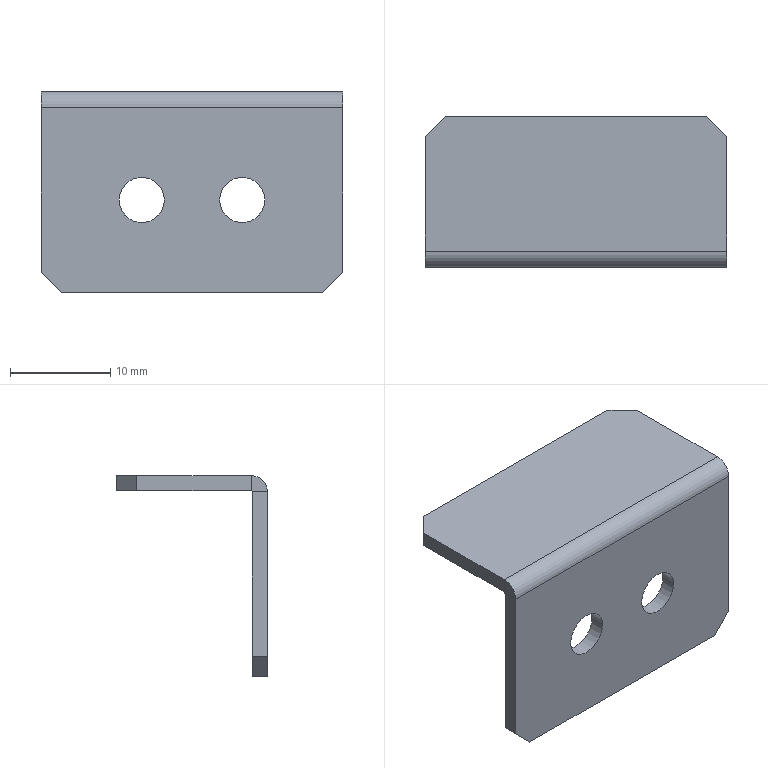Part | SolidWorks | features Chamfer 1, ICE 1, SplitBody 1 | 1 solid | 22 faces | box 30 x 15 x 20 mm | volume 1431 mm3 | plane 16 | cylinder 6 | commonest cylinder face diameters 4.5 x4 0.2 x1 3.2 x1
STEP:
#1=CARTESIAN_POINT('',(23.95,17.2,288.));
#2=VERTEX_POINT('',#1);
#3=CARTESIAN_POINT('',(19.45,17.2,288.));
#4=VERTEX_POINT('',#3);
#5=CARTESIAN_POINT('',(21.7,17.2,288.));
#6=DIRECTION('',(0.,1.,0.));
#7=DIRECTION('',(-1.,0.,0.));
#8=AXIS2_PLACEMENT_3D('',#5,#6,#7);
#9=CIRCLE('',#8,2.25);
#10=EDGE_CURVE('',#2,#4,#9,.T.);
#11=ORIENTED_EDGE('',*,*,#10,.F.);
#12=CARTESIAN_POINT('',(23.95,18.7,288.));
#13=VERTEX_POINT('',#12);
#14=CARTESIAN_POINT('',(23.95,8.7,288.));
#15=DIRECTION('',(0.,1.,0.));
#16=VECTOR('',#15,1000.);
#17=LINE('',#14,#16);
#18=EDGE_CURVE('',#2,#13,#17,.T.);
#19=ORIENTED_EDGE('',*,*,#18,.T.);
#20=CARTESIAN_POINT('',(19.45,18.7,288.));
#21=VERTEX_POINT('',#20);
#22=CARTESIAN_POINT('',(21.7,18.7,288.));
#23=DIRECTION('',(0.,1.,0.));
#24=DIRECTION('',(-1.,0.,0.));
#25=AXIS2_PLACEMENT_3D('',#22,#23,#24);
#26=CIRCLE('',#25,2.25);
#27=EDGE_CURVE('',#13,#21,#26,.T.);
#28=ORIENTED_EDGE('',*,*,#27,.T.);
#29=CARTESIAN_POINT('',(19.45,8.7,288.));
#30=DIRECTION('',(0.,1.,0.));
#31=VECTOR('',#30,1000.);
#32=LINE('',#29,#31);
#33=EDGE_CURVE('',#4,#21,#32,.T.);
#34=ORIENTED_EDGE('',*,*,#33,.F.);
#35=EDGE_LOOP('',(#11,#19,#28,#34));
#36=FACE_OUTER_BOUND('',#35,.T.);
#37=CARTESIAN_POINT('',(21.7,8.7,288.));
#38=DIRECTION('',(0.,1.,0.));
#39=DIRECTION('',(-1.,0.,0.));
#40=AXIS2_PLACEMENT_3D('',#37,#38,#39);
#41=CYLINDRICAL_SURFACE('',#40,2.25);
#42=ADVANCED_FACE('',(#36),#41,.F.);
#43=CARTESIAN_POINT('',(13.95,18.7,288.));
#44=VERTEX_POINT('',#43);
#45=CARTESIAN_POINT('',(9.45,18.7,288.));
#46=VERTEX_POINT('',#45);
#47=CARTESIAN_POINT('',(11.7,18.7,288.));
#48=DIRECTION('',(0.,-1.,0.));
#49=DIRECTION('',(1.,0.,0.));
#50=AXIS2_PLACEMENT_3D('',#47,#48,#49);
#51=CIRCLE('',#50,2.25);
#52=EDGE_CURVE('',#44,#46,#51,.T.);
#53=ORIENTED_EDGE('',*,*,#52,.F.);
#54=CARTESIAN_POINT('',(13.95,17.2,288.));
#55=VERTEX_POINT('',#54);
#56=CARTESIAN_POINT('',(13.95,22.2,288.));
#57=DIRECTION('',(0.,-1.,0.));
#58=VECTOR('',#57,1000.);
#59=LINE('',#56,#58);
#60=EDGE_CURVE('',#44,#55,#59,.T.);
#61=ORIENTED_EDGE('',*,*,#60,.T.);
#62=CARTESIAN_POINT('',(9.45,17.2,288.));
#63=VERTEX_POINT('',#62);
#64=CARTESIAN_POINT('',(11.7,17.2,288.));
#65=DIRECTION('',(0.,1.,0.));
#66=DIRECTION('',(-1.,0.,0.));
#67=AXIS2_PLACEMENT_3D('',#64,#65,#66);
#68=CIRCLE('',#67,2.25);
#69=EDGE_CURVE('',#63,#55,#68,.T.);
#70=ORIENTED_EDGE('',*,*,#69,.F.);
#71=CARTESIAN_POINT('',(9.45,22.2,288.));
#72=DIRECTION('',(0.,-1.,0.));
#73=VECTOR('',#72,1000.);
#74=LINE('',#71,#73);
#75=EDGE_CURVE('',#46,#63,#74,.T.);
#76=ORIENTED_EDGE('',*,*,#75,.F.);
#77=EDGE_LOOP('',(#53,#61,#70,#76));
#78=FACE_OUTER_BOUND('',#77,.T.);
#79=CARTESIAN_POINT('',(11.7,22.2,288.));
#80=DIRECTION('',(0.,-1.,0.));
#81=DIRECTION('',(-1.,0.,0.));
#82=AXIS2_PLACEMENT_3D('',#79,#80,#81);
#83=CYLINDRICAL_SURFACE('',#82,2.25);
#84=ADVANCED_FACE('',(#78),#83,.F.);
#85=CARTESIAN_POINT('',(31.7,17.2,297.2));
#86=VERTEX_POINT('',#85);
#87=CARTESIAN_POINT('',(31.7,18.7,297.2));
#88=VERTEX_POINT('',#87);
#89=CARTESIAN_POINT('',(31.7,17.2,297.2));
#90=DIRECTION('',(0.,1.,0.));
#91=VECTOR('',#90,1000.);
#92=LINE('',#89,#91);
#93=EDGE_CURVE('',#86,#88,#92,.T.);
#94=ORIENTED_EDGE('',*,*,#93,.T.);
#95=CARTESIAN_POINT('',(31.7,18.8,297.3));
#96=VERTEX_POINT('',#95);
#97=CARTESIAN_POINT('',(31.7,18.8,297.2));
#98=DIRECTION('',(-1.,0.,0.));
#99=DIRECTION('',(0.,0.,-1.));
#100=AXIS2_PLACEMENT_3D('',#97,#98,#99);
#101=CIRCLE('',#100,0.1);
#102=EDGE_CURVE('',#88,#96,#101,.T.);
#103=ORIENTED_EDGE('',*,*,#102,.T.);
#104=CARTESIAN_POINT('',(31.7,18.8,298.8));
#105=VERTEX_POINT('',#104);
#106=CARTESIAN_POINT('',(31.7,18.8,297.3));
#107=DIRECTION('',(0.,0.,1.));
#108=VECTOR('',#107,1000.);
#109=LINE('',#106,#108);
#110=EDGE_CURVE('',#96,#105,#109,.T.);
#111=ORIENTED_EDGE('',*,*,#110,.T.);
#112=CARTESIAN_POINT('',(31.7,18.8,297.2));
#113=DIRECTION('',(-1.,0.,0.));
#114=DIRECTION('',(0.,1.,0.));
#115=AXIS2_PLACEMENT_3D('',#112,#113,#114);
#116=CIRCLE('',#115,1.6);
#117=EDGE_CURVE('',#86,#105,#116,.T.);
#118=ORIENTED_EDGE('',*,*,#117,.F.);
#119=EDGE_LOOP('',(#94,#103,#111,#118));
#120=FACE_OUTER_BOUND('',#119,.T.);
#121=CARTESIAN_POINT('',(31.7,17.2,297.2));
#122=DIRECTION('',(1.,0.,0.));
#123=DIRECTION('',(0.,-1.,0.));
#124=AXIS2_PLACEMENT_3D('',#121,#122,#123);
#125=PLANE('',#124);
#126=ADVANCED_FACE('',(#120),#125,.T.);
#127=CARTESIAN_POINT('',(31.7,17.2,280.8));
#128=VERTEX_POINT('',#127);
#129=CARTESIAN_POINT('',(31.7,17.2,278.8));
#130=DIRECTION('',(0.,0.,1.));
#131=VECTOR('',#130,1000.);
#132=LINE('',#129,#131);
#133=EDGE_CURVE('',#128,#86,#132,.T.);
#134=ORIENTED_EDGE('',*,*,#133,.F.);
#135=CARTESIAN_POINT('',(31.7,18.7,280.8));
#136=VERTEX_POINT('',#135);
#137=CARTESIAN_POINT('',(31.7,18.8,280.8));
#138=DIRECTION('',(0.,1.,0.));
#139=VECTOR('',#138,1000.);
#140=LINE('',#137,#139);
#141=EDGE_CURVE('',#128,#136,#140,.T.);
#142=ORIENTED_EDGE('',*,*,#141,.T.);
#143=CARTESIAN_POINT('',(31.7,18.7,278.8));
#144=DIRECTION('',(0.,0.,1.));
#145=VECTOR('',#144,1000.);
#146=LINE('',#143,#145);
#147=EDGE_CURVE('',#136,#88,#146,.T.);
#148=ORIENTED_EDGE('',*,*,#147,.T.);
#149=ORIENTED_EDGE('',*,*,#93,.F.);
#150=EDGE_LOOP('',(#134,#142,#148,#149));
#151=FACE_OUTER_BOUND('',#150,.T.);
#152=CARTESIAN_POINT('',(31.7,18.8,297.3));
#153=DIRECTION('',(1.,0.,0.));
#154=DIRECTION('',(0.,-1.,0.));
#155=AXIS2_PLACEMENT_3D('',#152,#153,#154);
#156=PLANE('',#155);
#157=ADVANCED_FACE('',(#151),#156,.T.);
#158=CARTESIAN_POINT('',(1.7,18.8,298.8));
#159=VERTEX_POINT('',#158);
#160=CARTESIAN_POINT('',(1.7,18.8,297.3));
#161=VERTEX_POINT('',#160);
#162=CARTESIAN_POINT('',(1.7,18.8,298.8));
#163=DIRECTION('',(0.,0.,-1.));
#164=VECTOR('',#163,1000.);
#165=LINE('',#162,#164);
#166=EDGE_CURVE('',#159,#161,#165,.T.);
#167=ORIENTED_EDGE('',*,*,#166,.T.);
#168=CARTESIAN_POINT('',(1.7,18.7,297.2));
#169=VERTEX_POINT('',#168);
#170=CARTESIAN_POINT('',(1.7,18.8,297.2));
#171=DIRECTION('',(-1.,0.,0.));
#172=DIRECTION('',(0.,0.,-1.));
#173=AXIS2_PLACEMENT_3D('',#170,#171,#172);
#174=CIRCLE('',#173,0.1);
#175=EDGE_CURVE('',#169,#161,#174,.T.);
#176=ORIENTED_EDGE('',*,*,#175,.F.);
#177=CARTESIAN_POINT('',(1.7,17.2,297.2));
#178=VERTEX_POINT('',#177);
#179=CARTESIAN_POINT('',(1.7,18.7,297.2));
#180=DIRECTION('',(0.,-1.,0.));
#181=VECTOR('',#180,1000.);
#182=LINE('',#179,#181);
#183=EDGE_CURVE('',#169,#178,#182,.T.);
#184=ORIENTED_EDGE('',*,*,#183,.T.);
#185=CARTESIAN_POINT('',(1.7,18.8,297.2));
#186=DIRECTION('',(-1.,0.,0.));
#187=DIRECTION('',(0.,1.,0.));
#188=AXIS2_PLACEMENT_3D('',#185,#186,#187);
#189=CIRCLE('',#188,1.6);
#190=EDGE_CURVE('',#178,#159,#189,.T.);
#191=ORIENTED_EDGE('',*,*,#190,.T.);
#192=EDGE_LOOP('',(#167,#176,#184,#191));
#193=FACE_OUTER_BOUND('',#192,.T.);
#194=CARTESIAN_POINT('',(1.7,18.8,298.8));
#195=DIRECTION('',(-1.,0.,0.));
#196=DIRECTION('',(0.,1.,0.));
#197=AXIS2_PLACEMENT_3D('',#194,#195,#196);
#198=PLANE('',#197);
#199=ADVANCED_FACE('',(#193),#198,.T.);
#200=CARTESIAN_POINT('',(1.7,30.2,298.8));
#201=VERTEX_POINT('',#200);
#202=CARTESIAN_POINT('',(1.7,17.2,298.8));
#203=DIRECTION('',(0.,1.,0.));
#204=VECTOR('',#203,1000.);
#205=LINE('',#202,#204);
#206=EDGE_CURVE('',#159,#201,#205,.T.);
#207=ORIENTED_EDGE('',*,*,#206,.T.);
#208=CARTESIAN_POINT('',(1.7,30.2,297.3));
#209=VERTEX_POINT('',#208);
#210=CARTESIAN_POINT('',(1.7,30.2,297.2));
#211=DIRECTION('',(0.,0.,-1.));
#212=VECTOR('',#211,1000.);
#213=LINE('',#210,#212);
#214=EDGE_CURVE('',#201,#209,#213,.T.);
#215=ORIENTED_EDGE('',*,*,#214,.T.);
#216=CARTESIAN_POINT('',(1.7,17.2,297.3));
#217=DIRECTION('',(0.,1.,0.));
#218=VECTOR('',#217,1000.);
#219=LINE('',#216,#218);
#220=EDGE_CURVE('',#161,#209,#219,.T.);
#221=ORIENTED_EDGE('',*,*,#220,.F.);
#222=ORIENTED_EDGE('',*,*,#166,.F.);
#223=EDGE_LOOP('',(#207,#215,#221,#222));
#224=FACE_OUTER_BOUND('',#223,.T.);
#225=CARTESIAN_POINT('',(1.7,18.7,297.2));
#226=DIRECTION('',(-1.,0.,0.));
#227=DIRECTION('',(0.,1.,0.));
#228=AXIS2_PLACEMENT_3D('',#225,#226,#227);
#229=PLANE('',#228);
#230=ADVANCED_FACE('',(#224),#229,.T.);
#231=CARTESIAN_POINT('',(29.7,32.2,298.8));
#232=VERTEX_POINT('',#231);
#233=CARTESIAN_POINT('',(3.7,32.2,298.8));
#234=VERTEX_POINT('',#233);
#235=CARTESIAN_POINT('',(31.7,32.2,298.8));
#236=DIRECTION('',(-1.,0.,0.));
#237=VECTOR('',#236,1000.);
#238=LINE('',#235,#237);
#239=EDGE_CURVE('',#232,#234,#238,.T.);
#240=ORIENTED_EDGE('',*,*,#239,.T.);
#241=CARTESIAN_POINT('',(3.7,32.2,298.8));
#242=DIRECTION('',(-0.7071,-0.7071,0.));
#243=VECTOR('',#242,1000.);
#244=LINE('',#241,#243);
#245=EDGE_CURVE('',#234,#201,#244,.T.);
#246=ORIENTED_EDGE('',*,*,#245,.T.);
#247=ORIENTED_EDGE('',*,*,#206,.F.);
#248=CARTESIAN_POINT('',(31.7,18.8,298.8));
#249=DIRECTION('',(-1.,0.,0.));
#250=VECTOR('',#249,1000.);
#251=LINE('',#248,#250);
#252=EDGE_CURVE('',#105,#159,#251,.T.);
#253=ORIENTED_EDGE('',*,*,#252,.F.);
#254=CARTESIAN_POINT('',(31.7,30.2,298.8));
#255=VERTEX_POINT('',#254);
#256=CARTESIAN_POINT('',(31.7,17.2,298.8));
#257=DIRECTION('',(0.,1.,0.));
#258=VECTOR('',#257,1000.);
#259=LINE('',#256,#258);
#260=EDGE_CURVE('',#105,#255,#259,.T.);
#261=ORIENTED_EDGE('',*,*,#260,.T.);
#262=CARTESIAN_POINT('',(31.7,30.2,298.8));
#263=DIRECTION('',(-0.7071,0.7071,0.));
#264=VECTOR('',#263,1000.);
#265=LINE('',#262,#264);
#266=EDGE_CURVE('',#255,#232,#265,.T.);
#267=ORIENTED_EDGE('',*,*,#266,.T.);
#268=EDGE_LOOP('',(#240,#246,#247,#253,#261,#267));
#269=FACE_OUTER_BOUND('',#268,.T.);
#270=CARTESIAN_POINT('',(31.7,17.2,298.8));
#271=DIRECTION('',(0.,0.,-1.));
#272=DIRECTION('',(-1.,0.,0.));
#273=AXIS2_PLACEMENT_3D('',#270,#271,#272);
#274=PLANE('',#273);
#275=ADVANCED_FACE('',(#269),#274,.F.);
#276=CARTESIAN_POINT('',(29.7,32.2,297.3));
#277=VERTEX_POINT('',#276);
#278=CARTESIAN_POINT('',(3.7,32.2,297.3));
#279=VERTEX_POINT('',#278);
#280=CARTESIAN_POINT('',(31.7,32.2,297.3));
#281=DIRECTION('',(-1.,0.,0.));
#282=VECTOR('',#281,1000.);
#283=LINE('',#280,#282);
#284=EDGE_CURVE('',#277,#279,#283,.T.);
#285=ORIENTED_EDGE('',*,*,#284,.T.);
#286=CARTESIAN_POINT('',(3.7,32.2,297.3));
#287=DIRECTION('',(0.,0.,1.));
#288=VECTOR('',#287,1000.);
#289=LINE('',#286,#288);
#290=EDGE_CURVE('',#279,#234,#289,.T.);
#291=ORIENTED_EDGE('',*,*,#290,.T.);
#292=ORIENTED_EDGE('',*,*,#239,.F.);
#293=CARTESIAN_POINT('',(29.7,32.2,297.3));
#294=DIRECTION('',(0.,0.,-1.));
#295=VECTOR('',#294,1000.);
#296=LINE('',#293,#295);
#297=EDGE_CURVE('',#232,#277,#296,.T.);
#298=ORIENTED_EDGE('',*,*,#297,.T.);
#299=EDGE_LOOP('',(#285,#291,#292,#298));
#300=FACE_OUTER_BOUND('',#299,.T.);
#301=CARTESIAN_POINT('',(31.7,32.2,297.3));
#302=DIRECTION('',(0.,1.,0.));
#303=DIRECTION('',(1.,0.,0.));
#304=AXIS2_PLACEMENT_3D('',#301,#302,#303);
#305=PLANE('',#304);
#306=ADVANCED_FACE('',(#300),#305,.T.);
#307=ORIENTED_EDGE('',*,*,#220,.T.);
#308=CARTESIAN_POINT('',(10.2,38.7,297.3));
#309=DIRECTION('',(0.7071,0.7071,0.));
#310=VECTOR('',#309,1000.);
#311=LINE('',#308,#310);
#312=EDGE_CURVE('',#209,#279,#311,.T.);
#313=ORIENTED_EDGE('',*,*,#312,.T.);
#314=ORIENTED_EDGE('',*,*,#284,.F.);
#315=CARTESIAN_POINT('',(31.7,30.2,297.3));
#316=VERTEX_POINT('',#315);
#317=CARTESIAN_POINT('',(38.2,23.7,297.3));
#318=DIRECTION('',(0.7071,-0.7071,0.));
#319=VECTOR('',#318,1000.);
#320=LINE('',#317,#319);
#321=EDGE_CURVE('',#277,#316,#320,.T.);
#322=ORIENTED_EDGE('',*,*,#321,.T.);
#323=CARTESIAN_POINT('',(31.7,17.2,297.3));
#324=DIRECTION('',(0.,1.,0.));
#325=VECTOR('',#324,1000.);
#326=LINE('',#323,#325);
#327=EDGE_CURVE('',#96,#316,#326,.T.);
#328=ORIENTED_EDGE('',*,*,#327,.F.);
#329=CARTESIAN_POINT('',(31.7,18.8,297.3));
#330=DIRECTION('',(-1.,0.,0.));
#331=VECTOR('',#330,1000.);
#332=LINE('',#329,#331);
#333=EDGE_CURVE('',#96,#161,#332,.T.);
#334=ORIENTED_EDGE('',*,*,#333,.T.);
#335=EDGE_LOOP('',(#307,#313,#314,#322,#328,#334));
#336=FACE_OUTER_BOUND('',#335,.T.);
#337=CARTESIAN_POINT('',(31.7,17.2,297.3));
#338=DIRECTION('',(0.,0.,-1.));
#339=DIRECTION('',(-1.,0.,0.));
#340=AXIS2_PLACEMENT_3D('',#337,#338,#339);
#341=PLANE('',#340);
#342=ADVANCED_FACE('',(#336),#341,.T.);
#343=ORIENTED_EDGE('',*,*,#175,.T.);
#344=ORIENTED_EDGE('',*,*,#333,.F.);
#345=ORIENTED_EDGE('',*,*,#102,.F.);
#346=CARTESIAN_POINT('',(31.7,18.7,297.2));
#347=DIRECTION('',(-1.,0.,0.));
#348=VECTOR('',#347,1000.);
#349=LINE('',#346,#348);
#350=EDGE_CURVE('',#88,#169,#349,.T.);
#351=ORIENTED_EDGE('',*,*,#350,.T.);
#352=EDGE_LOOP('',(#343,#344,#345,#351));
#353=FACE_OUTER_BOUND('',#352,.T.);
#354=CARTESIAN_POINT('',(31.7,18.8,297.2));
#355=DIRECTION('',(-1.,0.,0.));
#356=DIRECTION('',(0.,1.,0.));
#357=AXIS2_PLACEMENT_3D('',#354,#355,#356);
#358=CYLINDRICAL_SURFACE('',#357,0.1);
#359=ADVANCED_FACE('',(#353),#358,.F.);
#360=CARTESIAN_POINT('',(21.7,18.7,288.));
#361=DIRECTION('',(0.,1.,0.));
#362=DIRECTION('',(-1.,0.,0.));
#363=AXIS2_PLACEMENT_3D('',#360,#361,#362);
#364=CIRCLE('',#363,2.25);
#365=EDGE_CURVE('',#21,#13,#364,.T.);
#366=ORIENTED_EDGE('',*,*,#365,.F.);
#367=ORIENTED_EDGE('',*,*,#27,.F.);
#368=EDGE_LOOP('',(#366,#367));
#369=FACE_BOUND('',#368,.T.);
#370=CARTESIAN_POINT('',(11.7,18.7,288.));
#371=DIRECTION('',(0.,-1.,0.));
#372=DIRECTION('',(1.,0.,0.));
#373=AXIS2_PLACEMENT_3D('',#370,#371,#372);
#374=CIRCLE('',#373,2.25);
#375=EDGE_CURVE('',#46,#44,#374,.T.);
#376=ORIENTED_EDGE('',*,*,#375,.T.);
#377=ORIENTED_EDGE('',*,*,#52,.T.);
#378=EDGE_LOOP('',(#376,#377));
#379=FACE_BOUND('',#378,.T.);
#380=CARTESIAN_POINT('',(29.7,18.7,278.8));
#381=VERTEX_POINT('',#380);
#382=CARTESIAN_POINT('',(3.7,18.7,278.8));
#383=VERTEX_POINT('',#382);
#384=CARTESIAN_POINT('',(31.7,18.7,278.8));
#385=DIRECTION('',(-1.,0.,0.));
#386=VECTOR('',#385,1000.);
#387=LINE('',#384,#386);
#388=EDGE_CURVE('',#381,#383,#387,.T.);
#389=ORIENTED_EDGE('',*,*,#388,.T.);
#390=CARTESIAN_POINT('',(1.7,18.7,280.8));
#391=VERTEX_POINT('',#390);
#392=CARTESIAN_POINT('',(17.7,18.7,264.8));
#393=DIRECTION('',(-0.7071,0.,0.7071));
#394=VECTOR('',#393,1000.);
#395=LINE('',#392,#394);
#396=EDGE_CURVE('',#383,#391,#395,.T.);
#397=ORIENTED_EDGE('',*,*,#396,.T.);
#398=CARTESIAN_POINT('',(1.7,18.7,278.8));
#399=DIRECTION('',(0.,0.,1.));
#400=VECTOR('',#399,1000.);
#401=LINE('',#398,#400);
#402=EDGE_CURVE('',#391,#169,#401,.T.);
#403=ORIENTED_EDGE('',*,*,#402,.T.);
#404=ORIENTED_EDGE('',*,*,#350,.F.);
#405=ORIENTED_EDGE('',*,*,#147,.F.);
#406=CARTESIAN_POINT('',(30.7,18.7,279.8));
#407=DIRECTION('',(-0.7071,0.,-0.7071));
#408=VECTOR('',#407,1000.);
#409=LINE('',#406,#408);
#410=EDGE_CURVE('',#136,#381,#409,.T.);
#411=ORIENTED_EDGE('',*,*,#410,.T.);
#412=EDGE_LOOP('',(#389,#397,#403,#404,#405,#411));
#413=FACE_OUTER_BOUND('',#412,.T.);
#414=CARTESIAN_POINT('',(31.7,18.7,278.8));
#415=DIRECTION('',(0.,1.,0.));
#416=DIRECTION('',(1.,0.,0.));
#417=AXIS2_PLACEMENT_3D('',#414,#415,#416);
#418=PLANE('',#417);
#419=ADVANCED_FACE('',(#369,#379,#413),#418,.T.);
#420=CARTESIAN_POINT('',(29.7,17.2,278.8));
#421=VERTEX_POINT('',#420);
#422=CARTESIAN_POINT('',(3.7,17.2,278.8));
#423=VERTEX_POINT('',#422);
#424=CARTESIAN_POINT('',(31.7,17.2,278.8));
#425=DIRECTION('',(-1.,0.,0.));
#426=VECTOR('',#425,1000.);
#427=LINE('',#424,#426);
#428=EDGE_CURVE('',#421,#423,#427,.T.);
#429=ORIENTED_EDGE('',*,*,#428,.T.);
#430=CARTESIAN_POINT('',(3.7,18.7,278.8));
#431=DIRECTION('',(0.,1.,0.));
#432=VECTOR('',#431,1000.);
#433=LINE('',#430,#432);
#434=EDGE_CURVE('',#423,#383,#433,.T.);
#435=ORIENTED_EDGE('',*,*,#434,.T.);
#436=ORIENTED_EDGE('',*,*,#388,.F.);
#437=CARTESIAN_POINT('',(29.7,17.2,278.8));
#438=DIRECTION('',(0.,-1.,0.));
#439=VECTOR('',#438,1000.);
#440=LINE('',#437,#439);
#441=EDGE_CURVE('',#381,#421,#440,.T.);
#442=ORIENTED_EDGE('',*,*,#441,.T.);
#443=EDGE_LOOP('',(#429,#435,#436,#442));
#444=FACE_OUTER_BOUND('',#443,.T.);
#445=CARTESIAN_POINT('',(31.7,17.2,278.8));
#446=DIRECTION('',(0.,0.,-1.));
#447=DIRECTION('',(-1.,0.,0.));
#448=AXIS2_PLACEMENT_3D('',#445,#446,#447);
#449=PLANE('',#448);
#450=ADVANCED_FACE('',(#444),#449,.T.);
#451=CARTESIAN_POINT('',(21.7,17.2,288.));
#452=DIRECTION('',(0.,1.,0.));
#453=DIRECTION('',(-1.,0.,0.));
#454=AXIS2_PLACEMENT_3D('',#451,#452,#453);
#455=CIRCLE('',#454,2.25);
#456=EDGE_CURVE('',#4,#2,#455,.T.);
#457=ORIENTED_EDGE('',*,*,#456,.T.);
#458=ORIENTED_EDGE('',*,*,#10,.T.);
#459=EDGE_LOOP('',(#457,#458));
#460=FACE_BOUND('',#459,.T.);
#461=ORIENTED_EDGE('',*,*,#69,.T.);
#462=CARTESIAN_POINT('',(11.7,17.2,288.));
#463=DIRECTION('',(0.,1.,0.));
#464=DIRECTION('',(-1.,0.,0.));
#465=AXIS2_PLACEMENT_3D('',#462,#463,#464);
#466=CIRCLE('',#465,2.25);
#467=EDGE_CURVE('',#55,#63,#466,.T.);
#468=ORIENTED_EDGE('',*,*,#467,.T.);
#469=EDGE_LOOP('',(#461,#468));
#470=FACE_BOUND('',#469,.T.);
#471=CARTESIAN_POINT('',(1.7,17.2,280.8));
#472=VERTEX_POINT('',#471);
#473=CARTESIAN_POINT('',(1.7,17.2,278.8));
#474=DIRECTION('',(0.,0.,1.));
#475=VECTOR('',#474,1000.);
#476=LINE('',#473,#475);
#477=EDGE_CURVE('',#472,#178,#476,.T.);
#478=ORIENTED_EDGE('',*,*,#477,.F.);
#479=CARTESIAN_POINT('',(3.7,17.2,278.8));
#480=DIRECTION('',(0.7071,0.,-0.7071));
#481=VECTOR('',#480,1000.);
#482=LINE('',#479,#481);
#483=EDGE_CURVE('',#472,#423,#482,.T.);
#484=ORIENTED_EDGE('',*,*,#483,.T.);
#485=ORIENTED_EDGE('',*,*,#428,.F.);
#486=CARTESIAN_POINT('',(31.7,17.2,280.8));
#487=DIRECTION('',(0.7071,0.,0.7071));
#488=VECTOR('',#487,1000.);
#489=LINE('',#486,#488);
#490=EDGE_CURVE('',#421,#128,#489,.T.);
#491=ORIENTED_EDGE('',*,*,#490,.T.);
#492=ORIENTED_EDGE('',*,*,#133,.T.);
#493=CARTESIAN_POINT('',(31.7,17.2,297.2));
#494=DIRECTION('',(-1.,0.,0.));
#495=VECTOR('',#494,1000.);
#496=LINE('',#493,#495);
#497=EDGE_CURVE('',#86,#178,#496,.T.);
#498=ORIENTED_EDGE('',*,*,#497,.T.);
#499=EDGE_LOOP('',(#478,#484,#485,#491,#492,#498));
#500=FACE_OUTER_BOUND('',#499,.T.);
#501=CARTESIAN_POINT('',(31.7,17.2,278.8));
#502=DIRECTION('',(0.,1.,0.));
#503=DIRECTION('',(1.,0.,0.));
#504=AXIS2_PLACEMENT_3D('',#501,#502,#503);
#505=PLANE('',#504);
#506=ADVANCED_FACE('',(#460,#470,#500),#505,.F.);
#507=ORIENTED_EDGE('',*,*,#190,.F.);
#508=ORIENTED_EDGE('',*,*,#497,.F.);
#509=ORIENTED_EDGE('',*,*,#117,.T.);
#510=ORIENTED_EDGE('',*,*,#252,.T.);
#511=EDGE_LOOP('',(#507,#508,#509,#510));
#512=FACE_OUTER_BOUND('',#511,.T.);
#513=CARTESIAN_POINT('',(31.7,18.8,297.2));
#514=DIRECTION('',(-1.,0.,0.));
#515=DIRECTION('',(0.,1.,0.));
#516=AXIS2_PLACEMENT_3D('',#513,#514,#515);
#517=CYLINDRICAL_SURFACE('',#516,1.6);
#518=ADVANCED_FACE('',(#512),#517,.T.);
#519=ORIENTED_EDGE('',*,*,#327,.T.);
#520=CARTESIAN_POINT('',(31.7,30.2,297.2));
#521=DIRECTION('',(0.,0.,1.));
#522=VECTOR('',#521,1000.);
#523=LINE('',#520,#522);
#524=EDGE_CURVE('',#316,#255,#523,.T.);
#525=ORIENTED_EDGE('',*,*,#524,.T.);
#526=ORIENTED_EDGE('',*,*,#260,.F.);
#527=ORIENTED_EDGE('',*,*,#110,.F.);
#528=EDGE_LOOP('',(#519,#525,#526,#527));
#529=FACE_OUTER_BOUND('',#528,.T.);
#530=CARTESIAN_POINT('',(31.7,18.8,297.2));
#531=DIRECTION('',(1.,0.,0.));
#532=DIRECTION('',(0.,0.,-1.));
#533=AXIS2_PLACEMENT_3D('',#530,#531,#532);
#534=PLANE('',#533);
#535=ADVANCED_FACE('',(#529),#534,.T.);
#536=ORIENTED_EDGE('',*,*,#402,.F.);
#537=CARTESIAN_POINT('',(1.7,17.2,280.8));
#538=DIRECTION('',(0.,-1.,0.));
#539=VECTOR('',#538,1000.);
#540=LINE('',#537,#539);
#541=EDGE_CURVE('',#391,#472,#540,.T.);
#542=ORIENTED_EDGE('',*,*,#541,.T.);
#543=ORIENTED_EDGE('',*,*,#477,.T.);
#544=ORIENTED_EDGE('',*,*,#183,.F.);
#545=EDGE_LOOP('',(#536,#542,#543,#544));
#546=FACE_OUTER_BOUND('',#545,.T.);
#547=CARTESIAN_POINT('',(1.7,18.8,297.2));
#548=DIRECTION('',(1.,0.,0.));
#549=DIRECTION('',(0.,0.,-1.));
#550=AXIS2_PLACEMENT_3D('',#547,#548,#549);
#551=PLANE('',#550);
#552=ADVANCED_FACE('',(#546),#551,.F.);
#553=ORIENTED_EDGE('',*,*,#60,.F.);
#554=ORIENTED_EDGE('',*,*,#375,.F.);
#555=ORIENTED_EDGE('',*,*,#75,.T.);
#556=ORIENTED_EDGE('',*,*,#467,.F.);
#557=EDGE_LOOP('',(#553,#554,#555,#556));
#558=FACE_OUTER_BOUND('',#557,.T.);
#559=CARTESIAN_POINT('',(11.7,22.2,288.));
#560=DIRECTION('',(0.,-1.,0.));
#561=DIRECTION('',(-1.,0.,0.));
#562=AXIS2_PLACEMENT_3D('',#559,#560,#561);
#563=CYLINDRICAL_SURFACE('',#562,2.25);
#564=ADVANCED_FACE('',(#558),#563,.F.);
#565=ORIENTED_EDGE('',*,*,#483,.F.);
#566=ORIENTED_EDGE('',*,*,#541,.F.);
#567=ORIENTED_EDGE('',*,*,#396,.F.);
#568=ORIENTED_EDGE('',*,*,#434,.F.);
#569=EDGE_LOOP('',(#565,#566,#567,#568));
#570=FACE_OUTER_BOUND('',#569,.T.);
#571=CARTESIAN_POINT('',(3.7,17.2,278.8));
#572=DIRECTION('',(-0.7071,0.,-0.7071));
#573=DIRECTION('',(0.,-1.,0.));
#574=AXIS2_PLACEMENT_3D('',#571,#572,#573);
#575=PLANE('',#574);
#576=ADVANCED_FACE('',(#570),#575,.T.);
#577=ORIENTED_EDGE('',*,*,#312,.F.);
#578=ORIENTED_EDGE('',*,*,#214,.F.);
#579=ORIENTED_EDGE('',*,*,#245,.F.);
#580=ORIENTED_EDGE('',*,*,#290,.F.);
#581=EDGE_LOOP('',(#577,#578,#579,#580));
#582=FACE_OUTER_BOUND('',#581,.T.);
#583=CARTESIAN_POINT('',(3.7,32.2,297.3));
#584=DIRECTION('',(0.7071,-0.7071,0.));
#585=DIRECTION('',(0.,0.,1.));
#586=AXIS2_PLACEMENT_3D('',#583,#584,#585);
#587=PLANE('',#586);
#588=ADVANCED_FACE('',(#582),#587,.F.);
#589=ORIENTED_EDGE('',*,*,#321,.F.);
#590=ORIENTED_EDGE('',*,*,#297,.F.);
#591=ORIENTED_EDGE('',*,*,#266,.F.);
#592=ORIENTED_EDGE('',*,*,#524,.F.);
#593=EDGE_LOOP('',(#589,#590,#591,#592));
#594=FACE_OUTER_BOUND('',#593,.T.);
#595=CARTESIAN_POINT('',(31.7,30.2,297.2));
#596=DIRECTION('',(-0.7071,-0.7071,0.));
#597=DIRECTION('',(0.,0.,1.));
#598=AXIS2_PLACEMENT_3D('',#595,#596,#597);
#599=PLANE('',#598);
#600=ADVANCED_FACE('',(#594),#599,.F.);
#601=ORIENTED_EDGE('',*,*,#490,.F.);
#602=ORIENTED_EDGE('',*,*,#441,.F.);
#603=ORIENTED_EDGE('',*,*,#410,.F.);
#604=ORIENTED_EDGE('',*,*,#141,.F.);
#605=EDGE_LOOP('',(#601,#602,#603,#604));
#606=FACE_OUTER_BOUND('',#605,.T.);
#607=CARTESIAN_POINT('',(31.7,18.8,280.8));
#608=DIRECTION('',(-0.7071,0.,0.7071));
#609=DIRECTION('',(0.,1.,0.));
#610=AXIS2_PLACEMENT_3D('',#607,#608,#609);
#611=PLANE('',#610);
#612=ADVANCED_FACE('',(#606),#611,.F.);
#613=ORIENTED_EDGE('',*,*,#18,.F.);
#614=ORIENTED_EDGE('',*,*,#456,.F.);
#615=ORIENTED_EDGE('',*,*,#33,.T.);
#616=ORIENTED_EDGE('',*,*,#365,.T.);
#617=EDGE_LOOP('',(#613,#614,#615,#616));
#618=FACE_OUTER_BOUND('',#617,.T.);
#619=CARTESIAN_POINT('',(21.7,8.7,288.));
#620=DIRECTION('',(0.,1.,0.));
#621=DIRECTION('',(-1.,0.,0.));
#622=AXIS2_PLACEMENT_3D('',#619,#620,#621);
#623=CYLINDRICAL_SURFACE('',#622,2.25);
#624=ADVANCED_FACE('',(#618),#623,.F.);
#625=CLOSED_SHELL('',(#42,#84,#126,#157,#199,#230,#275,#306,#342,#359,#419,#450,#506,#518,#535,#552,#564,#576,#588,#600,#612,#624));
#626=MANIFOLD_SOLID_BREP('',#625);
#627=CARTESIAN_POINT('',(0.,0.,0.));
#628=DIRECTION('',(0.,0.,1.));
#629=DIRECTION('',(1.,0.,0.));
#630=AXIS2_PLACEMENT_3D('',#627,#628,#629);
#631=(LENGTH_UNIT()NAMED_UNIT(*)SI_UNIT(.MILLI.,.METRE.));
#632=UNCERTAINTY_MEASURE_WITH_UNIT(LENGTH_MEASURE(0.00001),#631,'','');
#633=(NAMED_UNIT(*)PLANE_ANGLE_UNIT()SI_UNIT($,.RADIAN.));
#634=(NAMED_UNIT(*)SI_UNIT($,.STERADIAN.)SOLID_ANGLE_UNIT());
#635=(GEOMETRIC_REPRESENTATION_CONTEXT(3)GLOBAL_UNCERTAINTY_ASSIGNED_CONTEXT((#632))GLOBAL_UNIT_ASSIGNED_CONTEXT((#631,#633,#634))REPRESENTATION_CONTEXT('',''));
#636=ADVANCED_BREP_SHAPE_REPRESENTATION('',(#626,#630),#635);